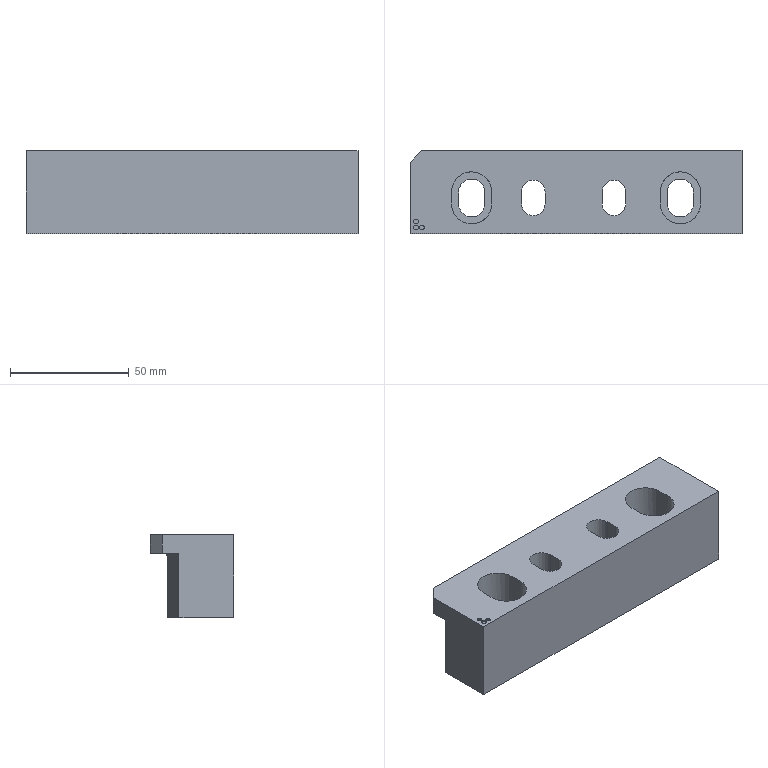Part | NX | features DIE-3 2 | 1 solid | 37 faces | box 140 x 35 x 35 mm | volume 119661 mm3 | plane 23 | cylinder 12 | spline 2 | commonest cylinder face diameters 2 x4 10 x4 11.007 x4